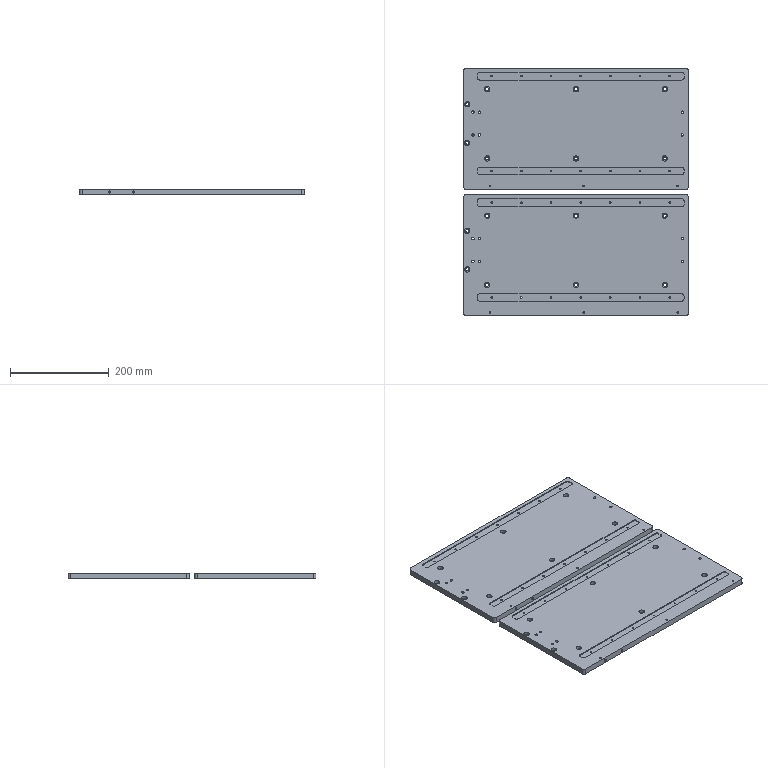CAM job | NX | 3-axis milling, drilling | part box 455 x 501 x 12 mm | stock box 460 x 506 x 12 mm
Tools:
number,name,description,diameter,corner_radius,flute_length,length,flutes
6,D6,平底铣刀-粗,6.0,0.0,25.0,75.0,2
9,D10,平底铣刀-粗,10.0,0.0,35.0,75.0,2
11,D2-J,平底铣刀-精,2.0,0.0,50.0,75.0,2
7,D6-J,平底铣刀-精,6.0,0.0,25.0,75.0,2
2,D6倒角刀,倒角刀,6.0,0.0,3.0,25.0,2
13,ZT3.3,钻头,3.3,0.0,35.0,50.0,2
15,ZT5,钻头,5.0,0.0,35.0,50.0,2
17,ZT6.5,钻头,6.5,0.0,35.0,50.0,2
13,钻头3.3,Twist Drill 3.3 mm,3.3,0.0,35.0,35.008,2
Operations:
program,operation,operation_type,tool,method,geometry_group,spindle_rpm,surface_speed,feed_per_tooth,feed_cut,feed_plunge,cut_length_mm,path_length_mm,cut_time_min,machine_time_min
A,SPOT,Operation,D6倒角刀,METHOD,W-A,3000.0,56.549,0.0333,200.0,0.0,155.0,3045.958,0.775,1.064
A,DRILL_HOLE,Operation,ZT3.3,METHOD,W-A,3500.0,35.186,0.0143,100.0,0.0,350.0,2689.524,3.5,3.734
A,DRILL_HOLE_2,Operation,钻头3.3,METHOD,W-A,3500.0,36.285,0.0143,100.0,0.0,75.0,1211.013,0.75,0.8636
A,DRILL_HOLE_3,Operation,ZT5,METHOD,W-A,2800.0,43.982,0.0214,120.0,0.0,150.0,1417.703,1.25,1.377
A,DRILL_HOLE_4,Operation,ZT6.5,METHOD,W-A,2500.0,51.051,0.03,150.0,0.0,200.0,2081.517,1.333,1.522
A,STEP_ROUGH_2,CavityMilling,D10,METHOD,W-A,6000.0,188.0,0.25,3500.0,100.0,13695.224,14672.755,3.945,4.043
A,HOLE_ROUGH_1,CylinderMilling,D6,METHOD,W-A,6000.0,113.097,0.1667,2000.0,100.0,3644.843,6049.052,1.822,2.063
A,PROFILE_ROUGH_2,VolumeBased25DMillingOperation,D10,METHOD,W-A,6000.0,188.0,0.25,4000.0,80.0,71176.013,71787.213,17.794,17.855
A,HOLE_SIDE_1,CylinderMilling,D6-J,METHOD,W-A,6000.0,113.097,0.0667,800.0,100.0,347.068,2860.077,0.4338,0.6851
A,FLOOR_FINISH_1,VolumeBased25DMillingOperation,D6-J,METHOD,W-A,6000.0,113.0,0.2083,1200.0,100.0,3399.437,3742.508,2.833,2.867
A,FLOOR_FINISH_2,VolumeBased25DMillingOperation,D6-J,METHOD,W-A,6000.0,113.0,0.2083,1200.0,100.0,3390.352,3741.645,2.825,2.86
A,FLOORWALL_SPIRAL_FINISH-M_COPY,VolumeBased25DMillingOperation,D2-J,SPIRAL_FINISH-DEPTHK-STEPG,W-A,8000.0,50.264,0.0375,600.0,100.0,4024.418,6550.141,6.707,6.96
A,FLOORWALL_SPIRAL_FINISH-M_COPY_COPY,VolumeBased25DMillingOperation,D2-J,SPIRAL_FINISH-DEPTHK-STEPG,W-A,8000.0,50.264,0.0375,600.0,100.0,4094.599,5772.151,6.824,6.992
A,FLOORWALL_SPIRAL_FINISH-M_COPY_COPY_COPY,VolumeBased25DMillingOperation,D2-J,SPIRAL_FINISH-DEPTHK-STEPG,W-A,8000.0,50.264,0.0375,600.0,100.0,3490.696,6868.997,5.818,6.156
A,SOLIDONLY,SurfaceContour,D6倒角刀,METHOD,W-A,6000.0,113.0,0.125,1200.0,100.0,6263.939,7140.351,5.22,5.308
A,DRILL_CHAMFER_1,Operation,D6倒角刀,METHOD,W-A,5000.0,94.248,0.015,150.0,0.0,144.2,2337.608,0.9613,1.181
A,DRILL_CHAMFER_2,Operation,D6倒角刀,METHOD,W-A,5000.0,94.248,0.015,150.0,0.0,31.2,1133.512,0.208,0.3182
A,MILL_CHAMFER_1,PlanarMilling,D6倒角刀,METHOD,W-A,6000.0,113.097,0.05,600.0,100.0,210.866,1783.988,0.3514,0.5088
A,MILL_CHAMFER_2,PlanarMilling,D6倒角刀,METHOD,W-A,6000.0,113.097,0.05,600.0,100.0,600.883,2883.771,1.002,1.23
A,FLOOR_SIDE_FINISH_3,VolumeBased25DMillingOperation,D6-J,METHOD,W-A,6000.0,113.0,0.2083,1200.0,100.0,1691.729,2033.721,1.41,1.444
A,FLOOR_SIDE_FINISH_4,VolumeBased25DMillingOperation,D6-J,METHOD,W-A,6000.0,113.0,0.2083,1200.0,100.0,1687.444,2036.325,1.406,1.441
A,PROFILE_SEMIFINISH_2,VolumeBased25DMillingOperation,D6-J,METHOD,W-A,6000.0,113.0,0.0833,1000.0,100.0,2830.503,3630.536,2.83,2.91
A,PROFILE_FINISH_2,VolumeBased25DMillingOperation,D6-J,METHOD,W-A,6000.0,113.0,0.0833,1000.0,100.0,2830.103,3631.182,2.83,2.91